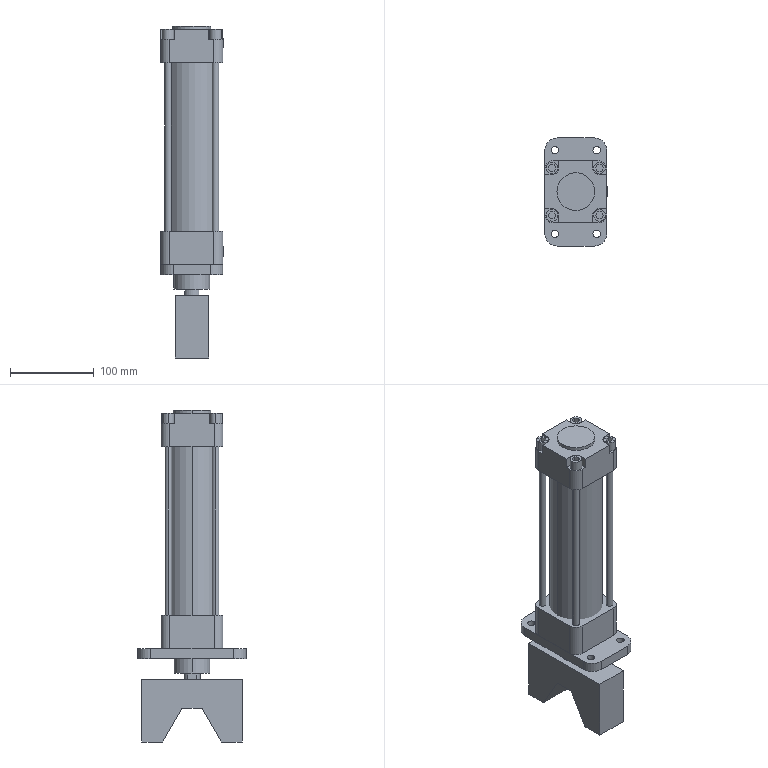Part | NX | 28 solids | 365 faces | box 74.5 x 129 x 396.319 mm | volume 982754 mm3 | plane 171 | cylinder 166 | cone 26 | spline 2 | commonest cylinder face diameters 16 x41 8 x24 14 x24 10 x12 9 x8 21.378 x8